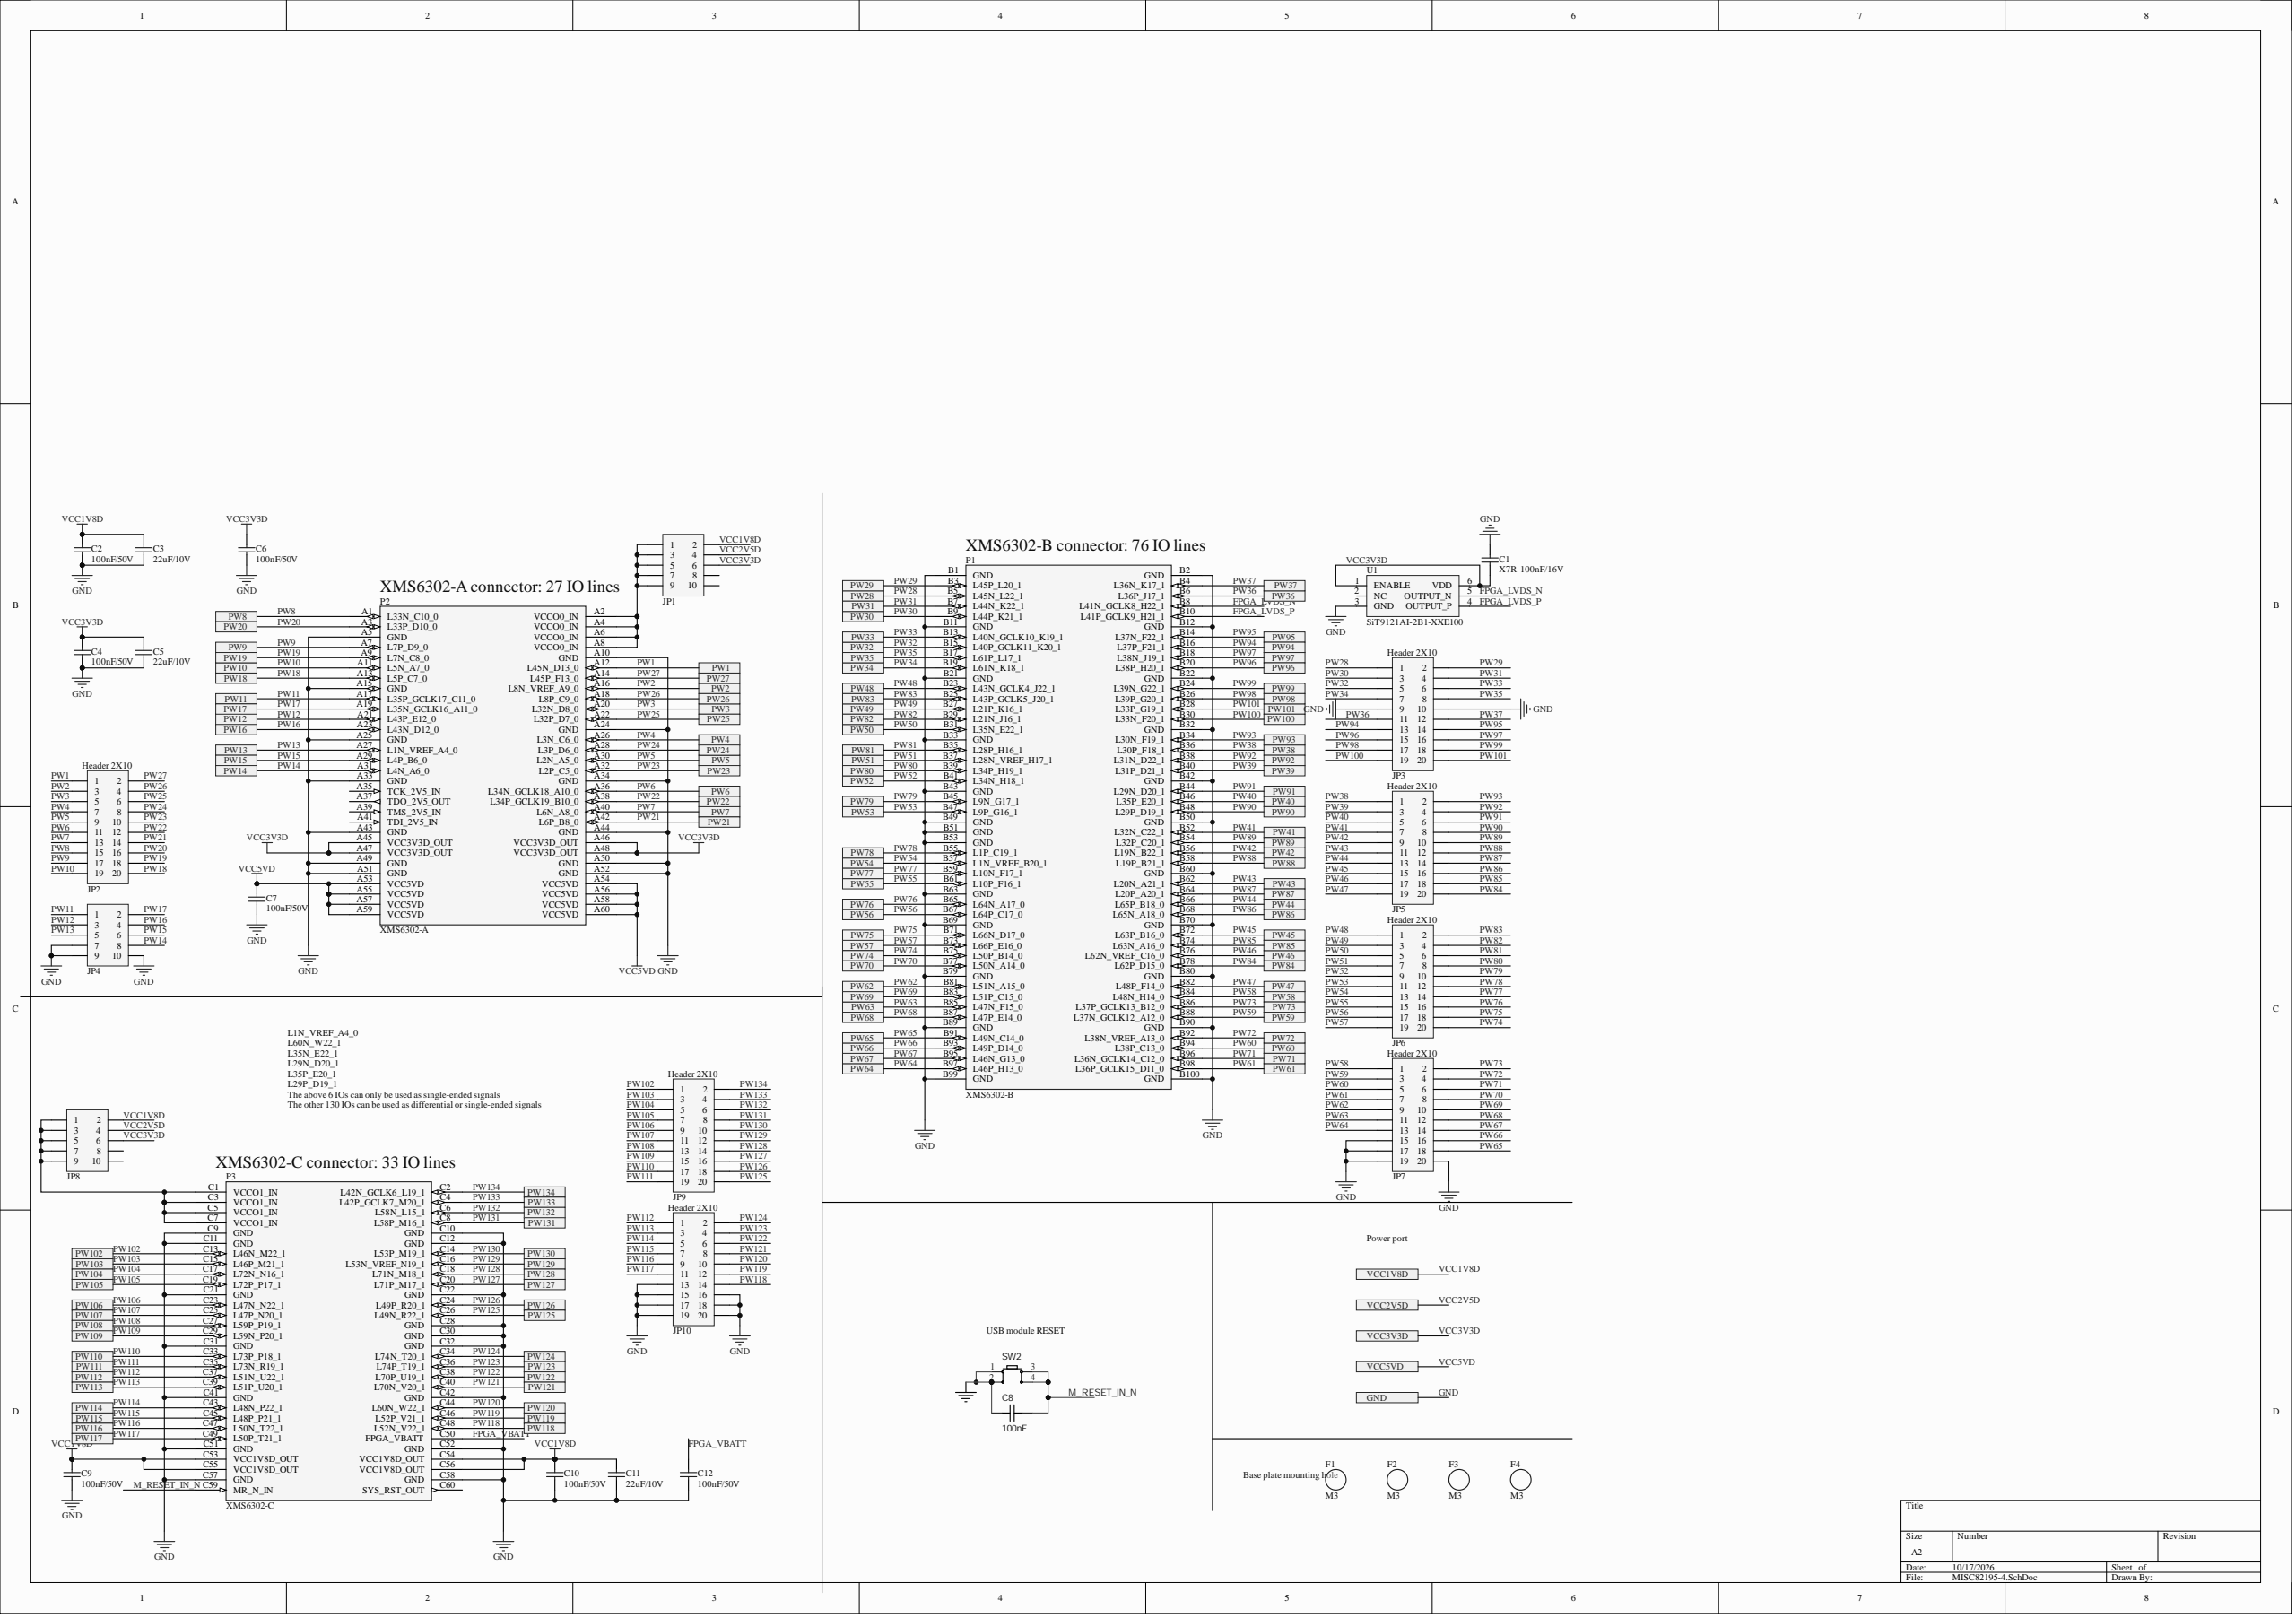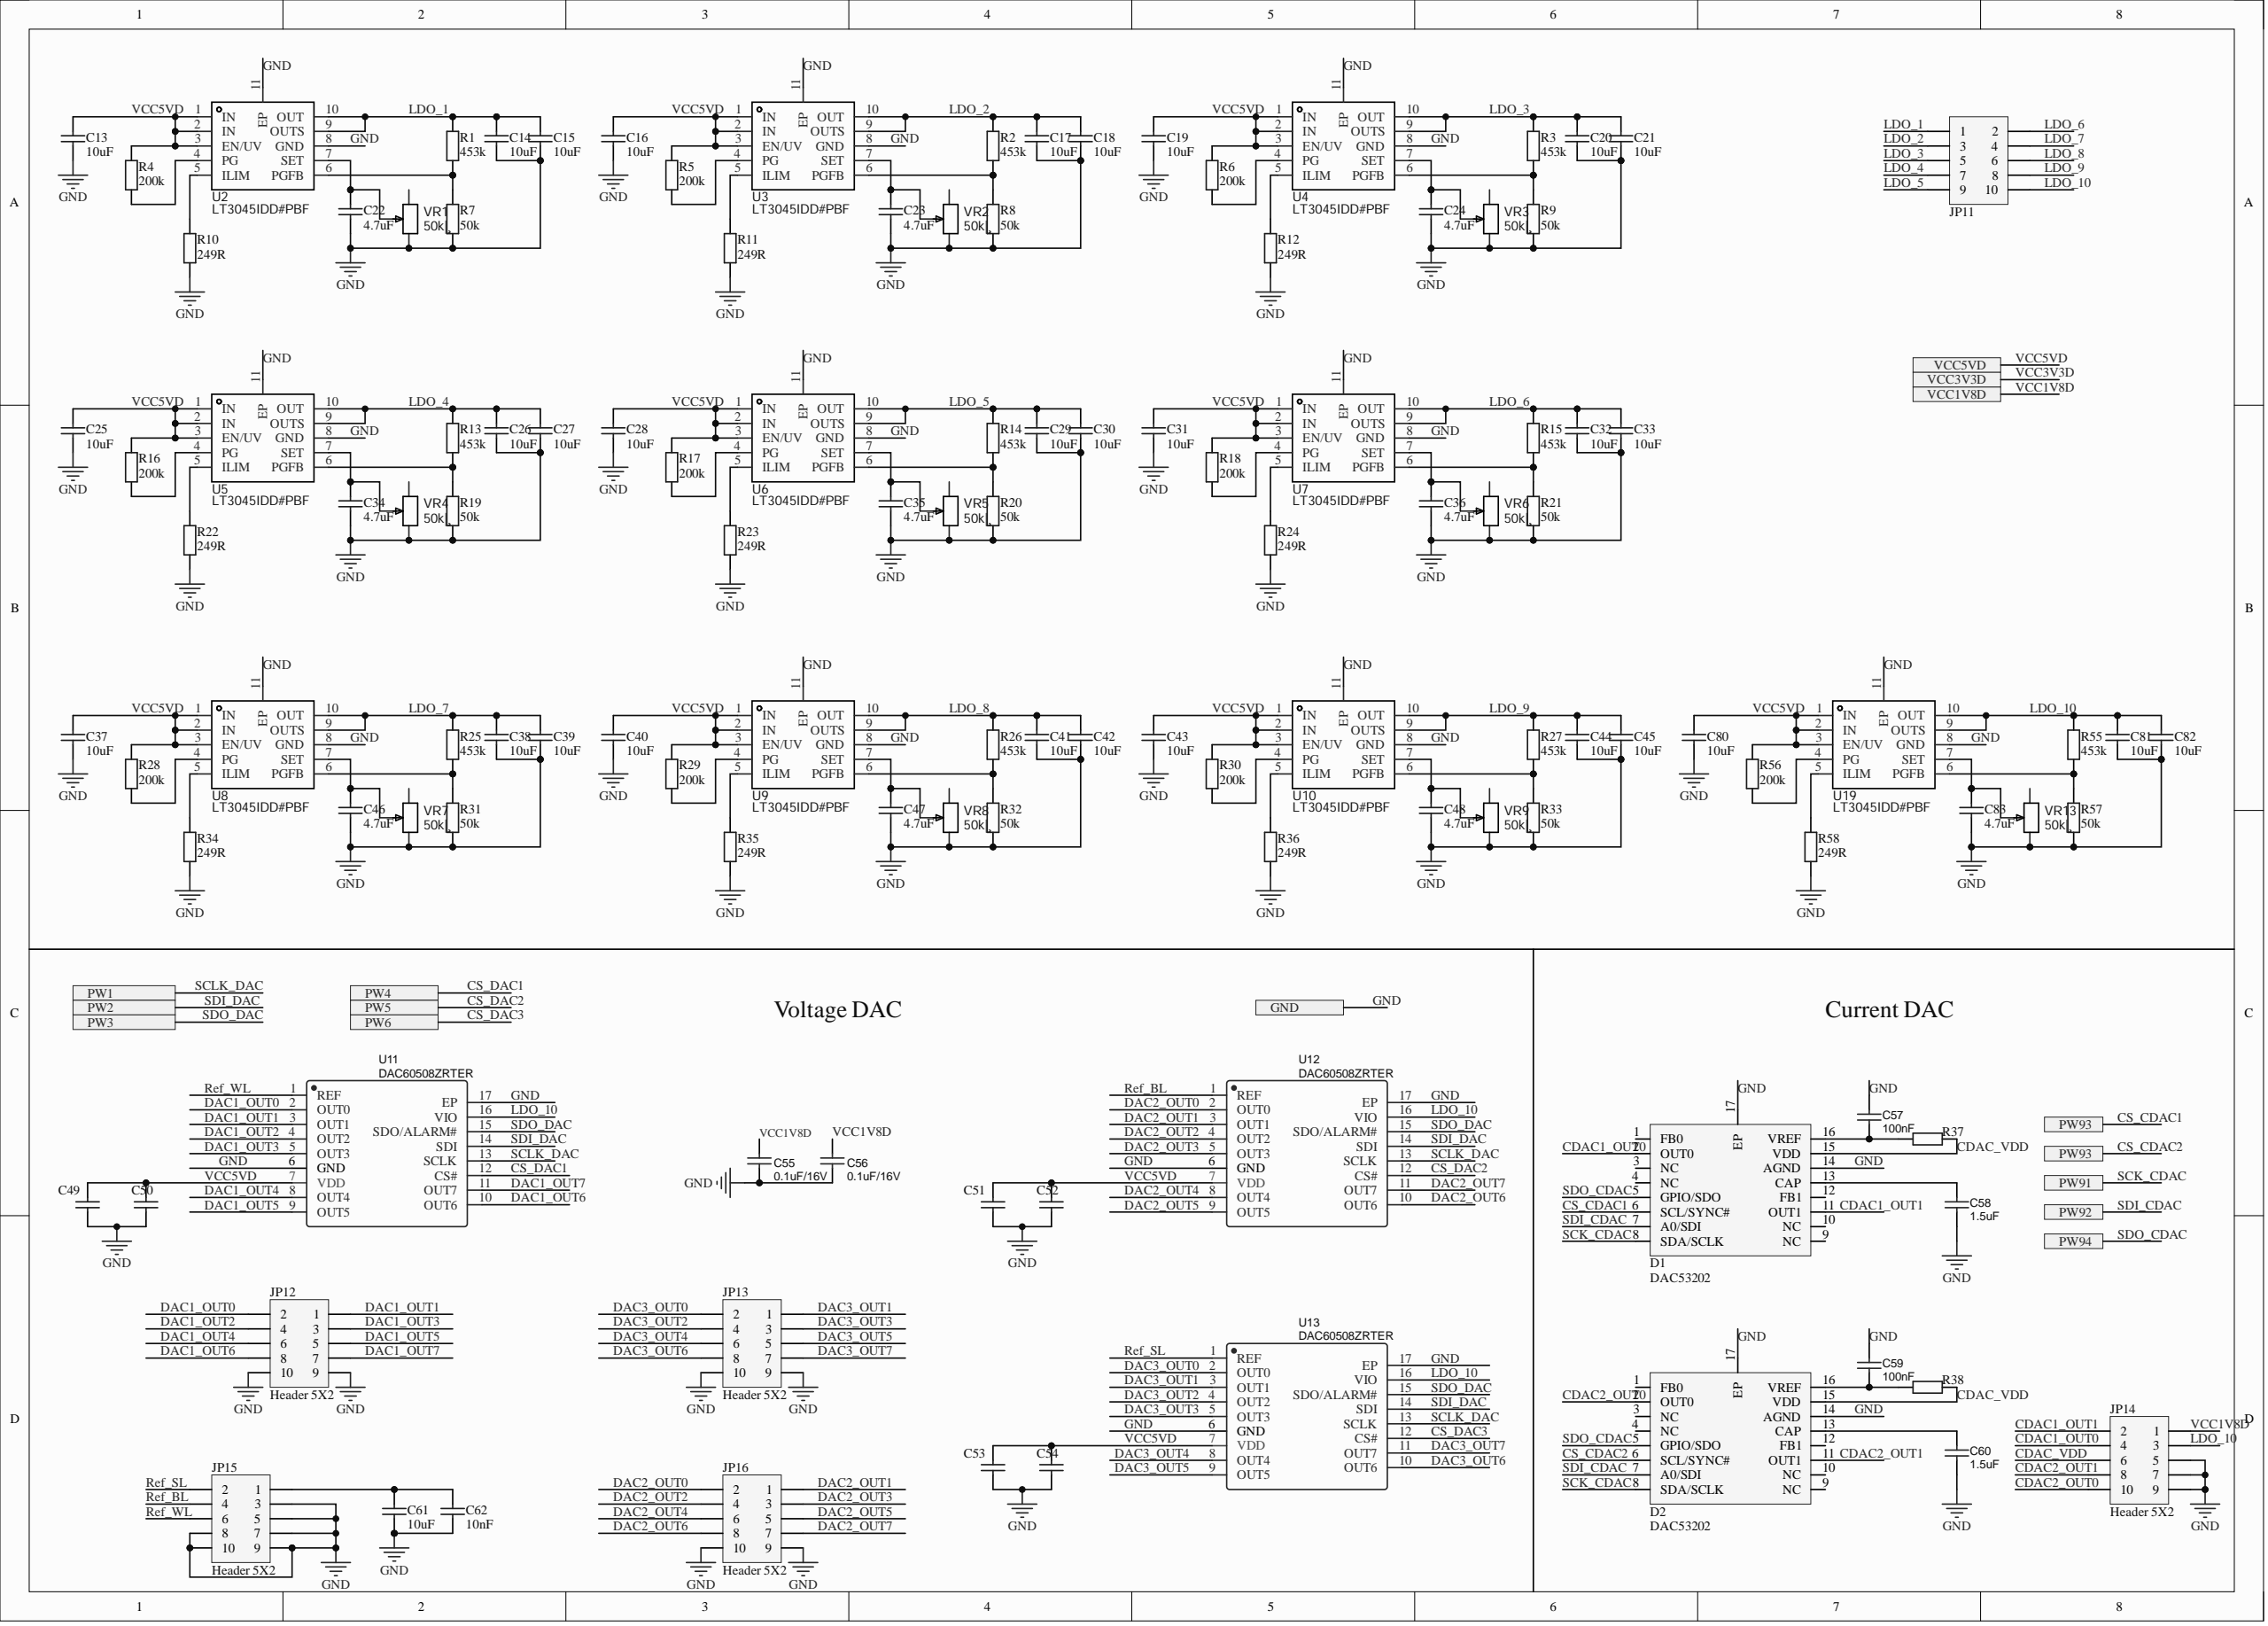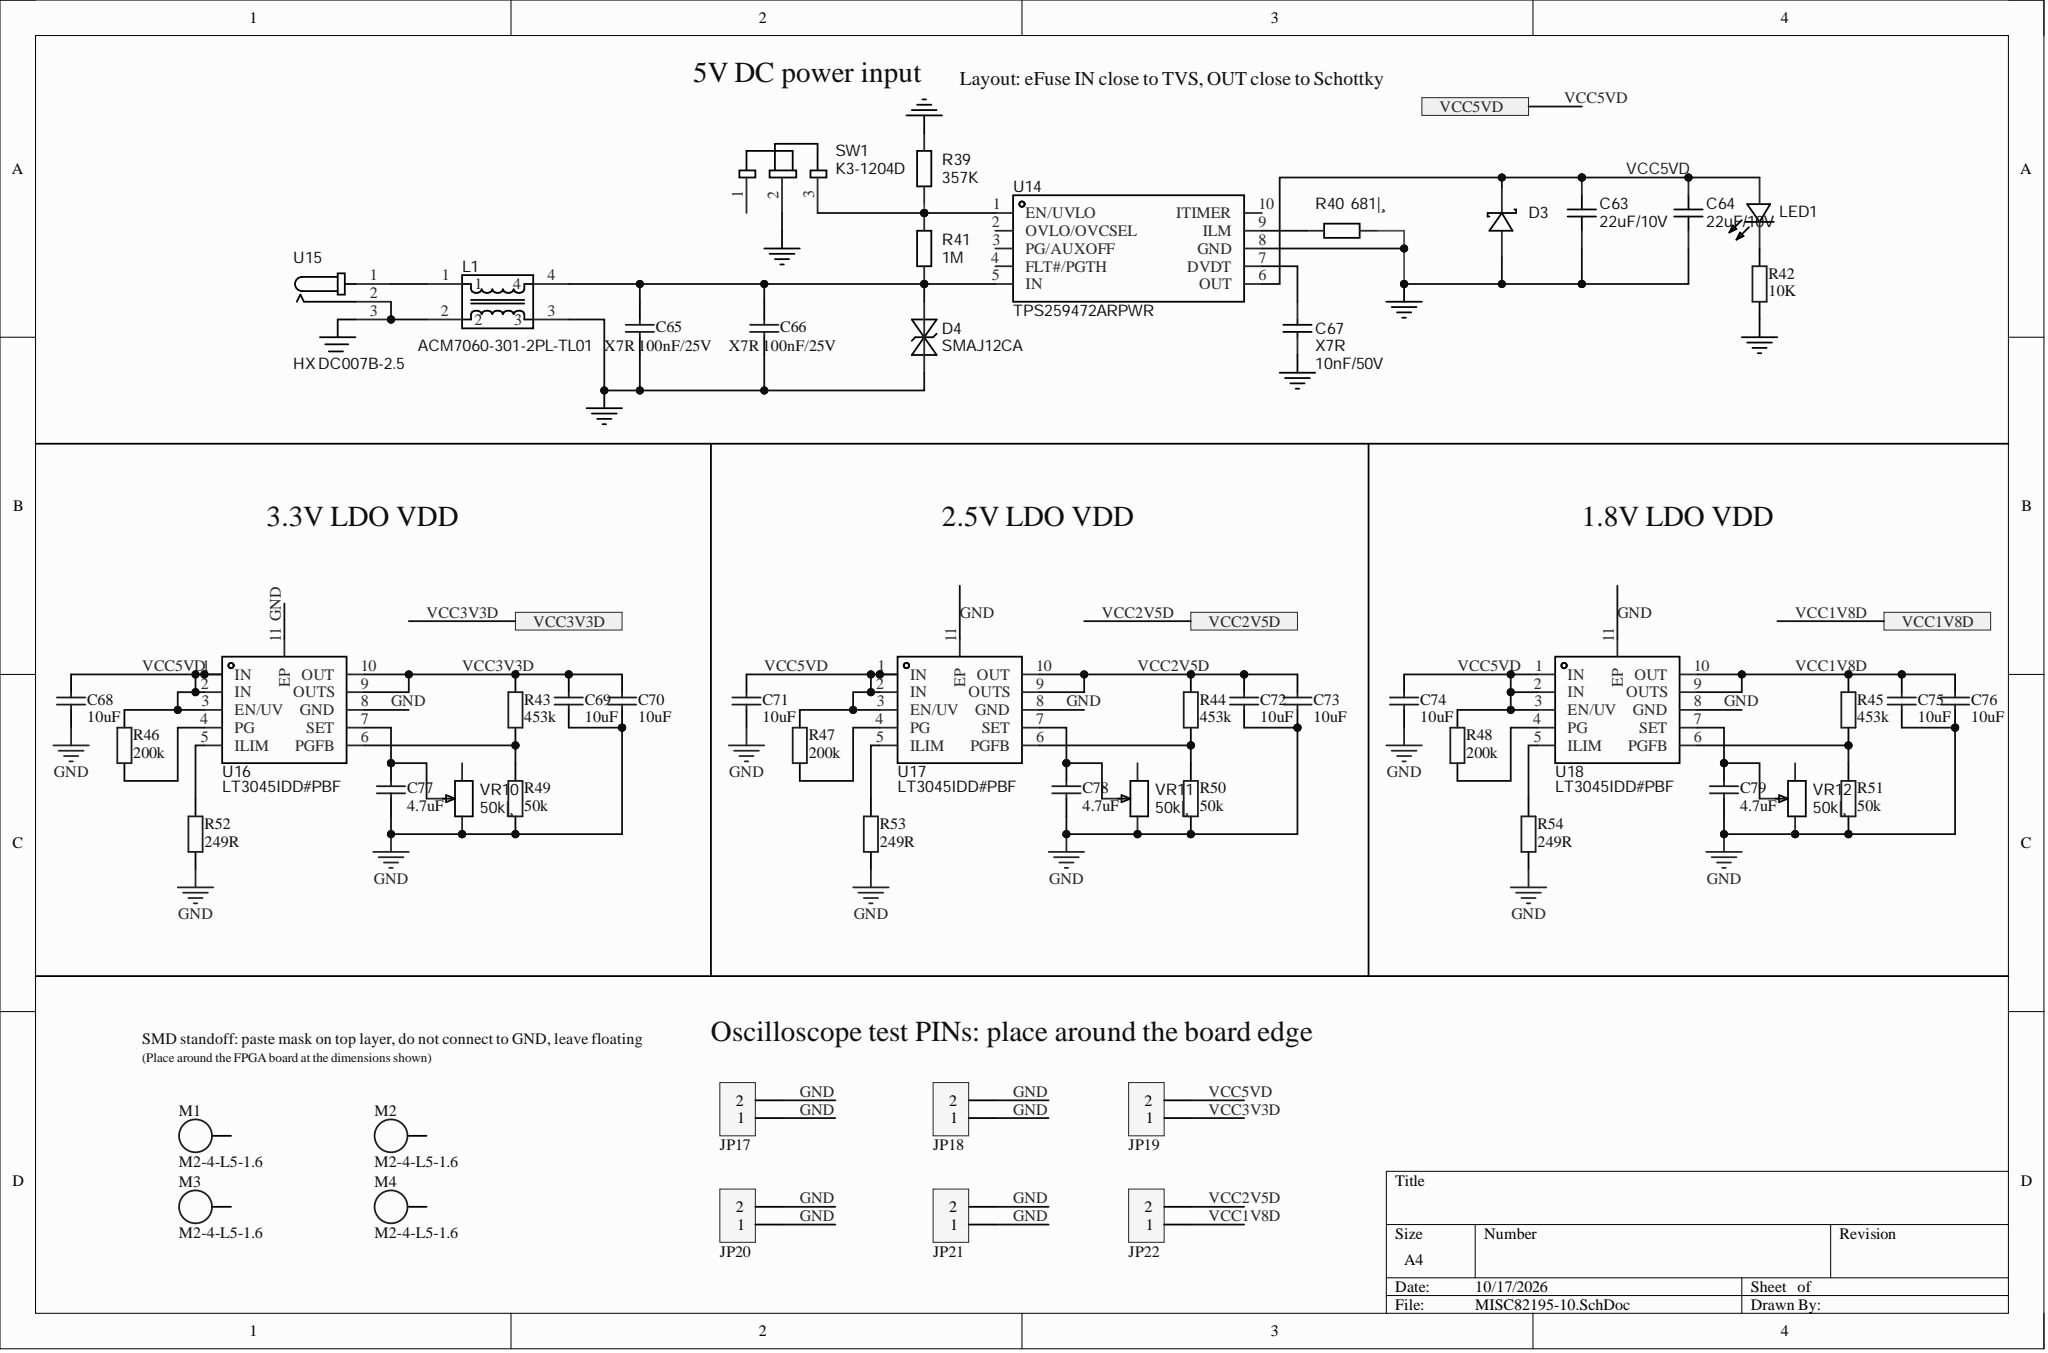Circuit board | Altium Designer | 214 parts | 251 nets
Bill of materials:
Comment,Description,Designator,Footprint,LibRef,Quantity
"X7R  100nF/16V","SMD capacitor","C1","C0603","C","1"
"100nF/50V","SMD capacitor","C2, C4, C6, C7, C9, C10, C12","C0603","C","7"
"22uF/10V","SMD capacitor, [NoValue]","C3, C5, C11, C63, C64","C0603","C, CL21A226MAQNNNE","5"
"100nF","[NoValue], SMD capacitor","C8, C50, C52, C54, C57, C59","C0603","CC0603KRX7R9BB104, C, 1uF","6"
"10uF","SMD capacitor","C13, C14, C15, C16, C17, C18, C19, C20, C21, C25, C26, C27, C28, C29, C30, C31, C32, C33, C37, C38, C39, C40, C41, C42, C43, C44, C45, C49, C51, C53, C61, C68, C69, C70, C71, C72, C73, C74, C75, C76, C80, C81, C82","C0603","C","43"
"4.7uF","SMD capacitor","C22, C23, C24, C34, C35, C36, C46, C47, C48, C77, C78, C79, C83","C0603","C","13"
"0.1uF/16V","","C55, C56","C0603","10nF","2"
"1.5uF","","C58, C60","C0603","1uF","2"
"10nF","SMD capacitor","C62","C0603","C","1"
"X7R 100nF/25V","SMD capacitor","C65, C66","C0603","C","2"
"X7R","","C67","C0603","CC0603KRX7R9BB103","1"
"DAC53202","","D1, D2","WQFN-16(3x3)","DAC53202","2"
"VS-10BQ015HM3/5BT","","D3","SMB_L4.6-W3.6-LS5.3-RD","VS-10BQ015HM3/5BT","1"
"SMAJ12CA","","D4","SMA_L4.2-W2.7-LS5.0-BI","SMAJ12CA_C908818","1"
"M3","Standoff hole","F1, F2, F3, F4","M3","M3","4"
"Header 5X2","5*2P connector","JP1, JP4, JP8, JP11, JP12, JP13, JP14, JP15, JP16","HDR2.54-LI-2x5P","Header 5X2","9"
"Header 2X10","10*2P connector","JP2, JP3, JP5, JP6, JP7, JP9, JP10","HDR2.54-LI-2x10P","Header 10X2","7"
"HDR-1X2","2P connector","JP17, JP18, JP19, JP20, JP21, JP22","HDR2.54-LI-2P","Header 2","6"
"ACM7060-301-2PL-TL01","","L1","FILTER-SMD_4P-L7.0-W6.0-TL_SMCM7060","ACM7060-301-2PL-TL01","1"
"NCD0805G1","","LED1","LED0805-R-RD","NCD0805G1","1"
"M2-4-L5-1.6","SMD standoff","M1, M2, M3, M4","M2.9","M2","4"
"XMS6302-B","","P1","XMS6302-B","XMS6302-B","1"
"XMS6302-A","","P2","XMS6302-A","XMS6302-A","1"
"XMS6302-C","","P3","XMS6302-C","XMS6302-C","1"
"453k","SMD resistor","R1, R2, R3, R13, R14, R15, R25, R26, R27, R43, R44, R45, R55","R0603","R","13"
"200k","SMD resistor","R4, R5, R6, R16, R17, R18, R28, R29, R30, R46, R47, R48, R56","R0603","R","13"
"50k","SMD resistor","R7, R8, R9, R19, R20, R21, R31, R32, R33, R49, R50, R51, R57","R0603","R","13"
"249R","SMD resistor","R10, R11, R12, R22, R23, R24, R34, R35, R36, R52, R53, R54, R58","R0603","R","13"
"10K","SMD resistor","R37, R38, R42","R0603","R","3"
"357K","","R39","R0603","Res_0603","1"
"681|¸","","R40","R0603","CR0805F681RP05Z","1"
"1M","","R41","R0603","Res_0603","1"
"K3-1204D","","SW1","SW-TH_K3-1204D","K3-1204D","1"
"Key_SMD_6x6x6.5","","SW2","SW-SMD_4P-L6.0-W6.0-P4.50-LS9.0-2","Key_SMD_6x6x6.5","1"
"SiT9121AI-2B1-XXE100","100MHz oscillator","U1","3225-6p","SiT9121AI","1"
"LT3045IDD#PBF","","U2, U3, U4, U5, U6, U7, U8, U9, U10, U16, U17, U18, U19","DFN-10_L3.0-W3.0-P0.50-BL-EP-3","LT3045IDD#PBF","13"
"DAC60508ZRTER","","U11, U12, U13","WQFN-16_L3.0-W3.0-P0.50-BL-EP0.8","DAC60508ZRTER","3"
"TPS259472ARPWR","","U14","VQFN-10_L2.0-W2.0-P0.45-TL","TPS259472ARPWR","1"
"HX DC007B-2.5","","U15","DC-IN-TH_HX-DC007B-2.5","HX DC007B-2.5","1"
"50k|¸","","VR1, VR2, VR3, VR4, VR5, VR6, VR7, VR8, VR9, VR10, VR11, VR12, VR13","RES-ADJ-SMD_3224W","3224W-1-503E","13"
Netlist (Protel format):
[
C1
C0603
X7R  100nF/16V



]
[
C2
C0603
100nF/50V



]
[
C3
C0603
22uF/10V



]
[
C4
C0603
100nF/50V



]
[
C5
C0603
22uF/10V



]
[
C6
C0603
100nF/50V



]
[
C7
C0603
100nF/50V



]
[
C8
C0603
100nF



]
[
C9
C0603
100nF/50V



]
[
C10
C0603
100nF/50V



]
[
C11
C0603
22uF/10V



]
[
C12
C0603
100nF/50V



]
[
C13
C0603
10uF



]
[
C14
C0603
10uF



]
[
C15
C0603
10uF



]
[
C16
C0603
10uF



]
[
C17
C0603
10uF



]
[
C18
C0603
10uF



]
[
C19
C0603
10uF



]
[
C20
C0603
10uF



]
[
C21
C0603
10uF



]
[
C22
C0603
4.7uF



]
[
C23
C0603
4.7uF



]
[
C24
C0603
4.7uF



]
[
C25
C0603
10uF



]
[
C26
C0603
10uF



]
[
C27
C0603
10uF



]
[
C28
C0603
10uF



]
[
C29
C0603
10uF



]
[
C30
C0603
10uF



]
[
C31
C0603
10uF



]
[
C32
C0603
10uF



]
[
C33
C0603
10uF



]
[
C34
C0603
4.7uF



]
[
C35
C0603
4.7uF



]
[
C36
C0603
4.7uF



]
[
C37
C0603
10uF



]
[
C38
C0603
10uF



]
[
C39
C0603
10uF



]
[
C40
C0603
10uF



]
[
C41
C0603
10uF



]
[
C42
C0603
10uF



]
[
C43
C0603
10uF



]
[
C44
C0603
10uF



]
[
C45
C0603
10uF



]
[
C46
C0603
4.7uF



]
[
C47
C0603
4.7uF



]
[
C48
C0603
4.7uF



]
[
C49
C0603
10uF



]
[
C50
C0603
100nF



]
[
C51
C0603
10uF



]
[
C52
C0603
100nF



]
[
C53
C0603
10uF



]
[
C54
C0603
100nF



]
[
C55
C0603
0.1uF/16V



]
[
C56
C0603
0.1uF/16V



]
[
C57
C0603
100nF



]
[
C58
C0603
1.5uF



]
[
C59
C0603
100nF



]
[
C60
C0603
1.5uF



]
[
C61
C0603
10uF



]
[
C62
C0603
10nF



]
[
C63
C0603
22uF/10V



]
[
C64
C0603
22uF/10V



]
[
C65
C0603
X7R 100nF/25V



]
[
C66
C0603
X7R 100nF/25V



]
[
C67
C0603
X7R



]
[
C68
C0603
10uF



]
[
C69
C0603
10uF



]
[
C70
C0603
10uF



]
[
C71
C0603
10uF



]
[
C72
C0603
10uF



]
[
C73
C0603
10uF



]
[
C74
C0603
10uF



]
[
C75
C0603
10uF



]
[
C76
C0603
10uF



]
[
C77
C0603
4.7uF



]
[
C78
C0603
4.7uF



]
[
C79
C0603
4.7uF



]
[
C80
C0603
10uF



]
[
C81
C0603
10uF



]
[
C82
C0603
10uF



]
[
C83
C0603
4.7uF



]
[
D1
WQFN-16(3x3)
DAC53202



]
[
D2
WQFN-16(3x3)
DAC53202



]
[
D3
SMB_L4.6-W3.6-LS5.3-RD
VS-10BQ015HM3/5BT



]
[
D4
SMA_L4.2-W2.7-LS5.0-BI
SMAJ12CA



]
[
F1
M3
M3



]
[
F2
M3
M3



]
[
F3
M3
M3



]
[
F4
M3
M3



]
[
JP1
HDR2.54-LI-2x5P
Header 5X2



]
[
JP2
HDR2.54-LI-2x10P
Header 2X10



]
[
JP3
HDR2.54-LI-2x10P
Header 2X10



]
[
JP4
HDR2.54-LI-2x5P
Header 5X2



]
[
JP5
HDR2.54-LI-2x10P
Header 2X10



]
[
JP6
HDR2.54-LI-2x10P
Header 2X10



]
[
JP7
HDR2.54-LI-2x10P
Header 2X10



]
[
JP8
HDR2.54-LI-2x5P
Header 5X2



]
[
JP9
HDR2.54-LI-2x10P
Header 2X10



]
[
JP10
HDR2.54-LI-2x10P
Header 2X10



]
[
JP11
HDR2.54-LI-2x5P
Header 5X2



]
[
JP12
HDR2.54-LI-2x5P
Header 5X2



]
[
JP13
HDR2.54-LI-2x5P
Header 5X2



]
[
JP14
HDR2.54-LI-2x5P
Header 5X2



]
[
JP15
HDR2.54-LI-2x5P
Header 5X2



]
[
JP16
HDR2.54-LI-2x5P
Header 5X2



]
[
JP17
HDR2.54-LI-2P
HDR-1X2



]
[
JP18
HDR2.54-LI-2P
HDR-1X2



]
[
JP19
HDR2.54-LI-2P
HDR-1X2



]
[
JP20
HDR2.54-LI-2P
HDR-1X2



]
[
JP21
HDR2.54-LI-2P
HDR-1X2



]
[
JP22
HDR2.54-LI-2P
HDR-1X2



]
[
L1
FILTER-SMD_4P-L7.0-W6.0-TL_SMCM7060
ACM7060-301-2PL-TL01



]
[
LED1
LED0805-R-RD
NCD0805G1



]
[
M1
M2.9
M2-4-L5-1.6



]
[
M2
M2.9
M2-4-L5-1.6



]
[
M3
M2.9
M2-4-L5-1.6



]
[
M4
M2.9
M2-4-L5-1.6



]
[
P1
XMS6302-B
XMS6302-B



]
[
P2
XMS6302-A
XMS6302-A



]
[
P3
XMS6302-C
XMS6302-C



]
[
R1
R0603
453k



]
[
R2
R0603
453k



]
[
R3
R0603
453k



]
[
R4
R0603
200k



]
[
R5
R0603
200k



]
[
R6
R0603
200k



]
[
R7
R0603
50k



]
[
R8
R0603
50k



]
[
R9
R0603
50k



]
[
R10
R0603
249R



]
[
R11
R0603
249R



]
[
R12
R0603
249R



]
[
R13
R0603
453k



]
[
R14
R0603
453k



]
[
R15
R0603
453k



]
[
R16
R0603
200k



]
[
R17
R0603
200k



]
[
R18
R0603
200k



]
[
R19
R0603
50k



]
[
R20
R0603
50k



]
[
R21
R0603
50k



]
[
R22
R0603
249R



]
[
R23
R0603
249R



]
[
R24
R0603
249R



]
[
R25
R0603
453k



]
[
R26
R0603
453k



]
[
R27
R0603
453k



]
[
R28
R0603
200k



]
[
R29
R0603
200k



]
[
R30
R0603
200k



]
[
R31
R0603
50k



]
[
R32
R0603
50k



]
[
R33
R0603
50k



]
[
R34
R0603
249R



]
[
R35
R0603
249R



]
[
R36
R0603
249R



]
[
R37
R0603
10K



]
[
R38
R0603
10K



]
[
R39
R0603
357K



]
[
R40
R0603
681|¸



]
[
R41
R0603
1M



]
[
R42
R0603
10K



]
[
R43
R0603
453k



]
[
R44
R0603
453k



]
[
R45
R0603
453k



]
[
R46
R0603
200k



]
[
R47
R0603
200k



]
[
R48
R0603
200k



]
[
R49
R0603
50k



]
[
R50
R0603
50k



]
[
R51
R0603
50k



]
[
R52
R0603
249R



]
[
R53
R0603
249R



]
[
R54
R0603
249R



]
[
R55
R0603
453k



]
[
R56
R0603
200k



]
[
R57
R0603
50k



]
[
R58
R0603
249R



]
[
SW1
SW-TH_K3-1204D
K3-1204D



]
[
SW2
SW-SMD_4P-L6.0-W6.0-P4.50-LS9.0-2
Key_SMD_6x6x6.5



]
[
U1
3225-6p
SiT9121AI-2B1-XXE100



]
[
U2
DFN-10_L3.0-W3.0-P0.50-BL-EP-3
LT3045IDD#PBF



]
[
U3
DFN-10_L3.0-W3.0-P0.50-BL-EP-3
LT3045IDD#PBF



]
[
U4
DFN-10_L3.0-W3.0-P0.50-BL-EP-3
LT3045IDD#PBF



]
[
U5
DFN-10_L3.0-W3.0-P0.50-BL-EP-3
LT3045IDD#PBF



]
[
U6
DFN-10_L3.0-W3.0-P0.50-BL-EP-3
LT3045IDD#PBF



]
[
U7
DFN-10_L3.0-W3.0-P0.50-BL-EP-3
LT3045IDD#PBF



]
[
U8
DFN-10_L3.0-W3.0-P0.50-BL-EP-3
LT3045IDD#PBF



]
[
U9
DFN-10_L3.0-W3.0-P0.50-BL-EP-3
LT3045IDD#PBF



]
[
U10
DFN-10_L3.0-W3.0-P0.50-BL-EP-3
LT3045IDD#PBF



]
[
U11
WQFN-16_L3.0-W3.0-P0.50-BL-EP0.8
DAC60508ZRTER



]
[
U12
WQFN-16_L3.0-W3.0-P0.50-BL-EP0.8
DAC60508ZRTER



]
[
U13
WQFN-16_L3.0-W3.0-P0.50-BL-EP0.8
DAC60508ZRTER



]
[
U14
VQFN-10_L2.0-W2.0-P0.45-TL
TPS259472ARPWR



]
[
U15
DC-IN-TH_HX-DC007B-2.5
HX DC007B-2.5



]
[
U16
DFN-10_L3.0-W3.0-P0.50-BL-EP-3
LT3045IDD#PBF



]
[
U17
DFN-10_L3.0-W3.0-P0.50-BL-EP-3
LT3045IDD#PBF



]
[
U18
DFN-10_L3.0-W3.0-P0.50-BL-EP-3
LT3045IDD#PBF



]
[
U19
DFN-10_L3.0-W3.0-P0.50-BL-EP-3
LT3045IDD#PBF



]
[
VR1
RES-ADJ-SMD_3224W
50k|¸



]
[
VR2
RES-ADJ-SMD_3224W
50k|¸



]
[
VR3
RES-ADJ-SMD_3224W
50k|¸



]
[
VR4
RES-ADJ-SMD_3224W
50k|¸



]
[
VR5
RES-ADJ-SMD_3224W
50k|¸



]
[
VR6
RES-ADJ-SMD_3224W
50k|¸



]
[
VR7
RES-ADJ-SMD_3224W
50k|¸



]
[
VR8
RES-ADJ-SMD_3224W
50k|¸



]
[
VR9
RES-ADJ-SMD_3224W
50k|¸



]
[
VR10
RES-ADJ-SMD_3224W
50k|¸



]
[
VR11
RES-ADJ-SMD_3224W
50k|¸



]
[
VR12
RES-ADJ-SMD_3224W
50k|¸



]
[
VR13
RES-ADJ-SMD_3224W
50k|¸



]
(
VCC5VD
C7-2
C13-2
C16-2
C19-2
C25-2
C28-2
C31-2
C37-2
C40-2
C43-2
C49-2
C50-2
C51-2
C52-2
C53-2
C54-2
C63-2
C64-2
C68-2
C71-2
C74-2
C80-2
D3-1
JP19-2
LED1-1
P2-A53
P2-A54
P2-A55
P2-A56
P2-A57
P2-A58
P2-A59
P2-A60
R4-2
R5-2
R6-2
R16-2
R17-2
R18-2
R28-2
R29-2
R30-2
R46-2
R47-2
R48-2
R56-2
U2-1
U2-2
U2-3
U3-1
U3-2
U3-3
U4-1
U4-2
U4-3
U5-1
U5-2
U5-3
U6-1
U6-2
U6-3
U7-1
U7-2
U7-3
U8-1
U8-2
U8-3
U9-1
U9-2
U9-3
U10-1
U10-2
U10-3
U11-7
U12-7
U13-7
U14-6
U16-1
U16-2
U16-3
U17-1
U17-2
U17-3
U18-1
U18-2
U18-3
U19-1
U19-2
U19-3
)
(
VCC3V3D
C1-1
C4-2
C5-2
C6-2
C69-2
C70-2
JP1-6
JP8-6
JP19-1
P2-A45
P2-A46
P2-A47
P2-A48
R43-2
U1-1
U1-6
U16-9
U16-10
)
(
VCC2V5D
C72-2
C73-2
JP1-4
JP8-4
JP22-2
R44-2
U17-9
U17-10
)
(
VCC1V8D
C2-2
C3-2
C9-2
C10-2
C11-2
C55-2
C56-2
C75-2
C76-2
JP1-2
JP8-2
JP14-1
JP22-1
P3-C53
P3-C54
P3-C55
P3-C56
R45-2
U18-9
U18-10
)
(
Ref_WL
JP15-6
U11-1
)
(
Ref_SL
JP15-2
U13-1
)
(
Ref_BL
JP15-4
U12-1
)
(
PW134
JP9-2
P3-C2
)
(
PW133
JP9-4
P3-C4
)
(
PW132
JP9-6
P3-C6
)
(
PW131
JP9-8
P3-C8
)
(
PW130
JP9-10
P3-C14
)
(
PW129
JP9-12
P3-C16
)
(
PW128
JP9-14
P3-C18
)
(
PW127
JP9-16
P3-C20
)
(
PW126
JP9-18
P3-C24
)
(
PW125
JP9-20
P3-C26
)
(
PW124
JP10-2
P3-C34
)
(
PW123
JP10-4
P3-C36
)
(
PW122
JP10-6
P3-C38
)
(
PW121
JP10-8
P3-C40
)
(
PW120
JP10-10
P3-C44
)
(
PW119
JP10-12
P3-C46
)
(
PW118
JP10-14
P3-C48
)
(
PW117
JP10-11
P3-C49
)
(
PW116
JP10-9
P3-C47
)
(
PW115
JP10-7
P3-C45
)
(
PW114
JP10-5
P3-C43
)
(
PW113
JP10-3
P3-C39
)
(
PW112
JP10-1
P3-C37
)
(
PW111
JP9-19
P3-C35
)
(
PW110
JP9-17
P3-C33
)
(
PW109
JP9-15
P3-C29
)
(
PW108
JP9-13
P3-C27
)
(
PW107
JP9-11
P3-C25
)
(
PW106
JP9-9
P3-C23
)
(
PW105
JP9-7
P3-C19
)
(
PW104
JP9-5
P3-C17
)
(
PW103
JP9-3
P3-C15
)
(
PW102
JP9-1
P3-C13
)
(
PW101
JP3-20
P1-B28
)
(
PW100
JP3-19
P1-B30
)
(
PW99
JP3-18
P1-B24
)
(
PW98
JP3-17
P1-B26
)
(
PW97
JP3-16
P1-B18
)
(
PW96
JP3-15
P1-B20
)
(
PW95
JP3-14
P1-B14
)
(
PW94
D1-5
D2-5
JP3-13
P1-B16
)
(
PW92
D1-7
D2-7
JP5-4
P1-B38
)
(
PW91
D1-8
D2-8
JP5-6
P1-B44
)
(
PW90
JP5-8
P1-B48
)
(
PW89
JP5-10
P1-B54
)
(
PW88
JP5-12
P1-B58
)
(
PW87
JP5-14
P1-B64
)
(
PW86
JP5-16
P1-B68
)
(
PW85
JP5-18
P1-B74
)
(
PW84
JP5-20
P1-B78
)
(
PW83
JP6-2
P1-B25
)
(
PW82
JP6-4
P1-B29
)
(
PW81
JP6-6
P1-B35
)
(
PW80
JP6-8
P1-B39
)
(
PW79
JP6-10
P1-B45
)
(
PW78
JP6-12
P1-B55
)
(
PW77
JP6-14
P1-B59
)
(
PW76
JP6-16
P1-B65
)
(
PW75
JP6-18
P1-B71
)
(
PW74
JP6-20
P1-B75
)
(
PW73
JP7-2
P1-B86
)
(
PW72
JP7-4
P1-B92
)
(
PW71
JP7-6
P1-B96
)
(
PW70
JP7-8
P1-B77
)
(
PW69
JP7-10
P1-B83
)
(
PW68
JP7-12
P1-B87
)
(
PW67
JP7-14
P1-B95
)
(
PW66
JP7-16
P1-B93
)
(
PW65
JP7-18
P1-B91
)
(
PW64
JP7-13
P1-B97
)
(
PW63
JP7-11
P1-B85
)
(
PW62
JP7-9
P1-B81
)
(
PW61
JP7-7
P1-B98
)
(
PW60
JP7-5
P1-B94
)
(
PW59
JP7-3
P1-B88
)
(
PW58
JP7-1
P1-B84
)
(
PW57
JP6-19
P1-B73
)
(
PW56
JP6-17
P1-B67
)
(
PW55
JP6-15
P1-B61
)
(
PW54
JP6-13
P1-B57
)
(
PW53
JP6-11
P1-B47
)
(
PW52
JP6-9
P1-B41
)
(
PW51
JP6-7
P1-B37
)
(
PW50
JP6-5
P1-B31
)
(
PW49
JP6-3
P1-B27
)
(
PW48
JP6-1
P1-B23
)
(
PW47
JP5-19
P1-B82
)
(
PW46
JP5-17
P1-B76
)
(
PW45
JP5-15
P1-B72
)
(
PW44
JP5-13
P1-B66
)
(
PW43
JP5-11
P1-B62
)
(
PW42
JP5-9
P1-B56
)
(
PW41
JP5-7
P1-B52
)
(
PW40
JP5-5
P1-B46
)
(
PW39
JP5-3
P1-B40
)
(
PW38
JP5-1
P1-B36
)
(
PW37
JP3-12
P1-B4
)
(
PW36
JP3-11
P1-B6
)
(
PW35
JP3-8
P1-B17
)
(
PW34
JP3-7
P1-B19
)
(
PW33
JP3-6
P1-B13
)
(
PW32
JP3-5
P1-B15
)
(
PW31
JP3-4
P1-B7
)
(
PW30
JP3-3
P1-B9
)
(
PW29
JP3-2
P1-B3
)
(
PW28
JP3-1
P1-B5
)
(
PW27
JP2-2
P2-A14
)
(
PW26
JP2-4
P2-A18
)
(
PW25
JP2-6
P2-A22
)
(
PW24
JP2-8
P2-A28
)
(
PW23
JP2-10
P2-A32
)
(
PW22
JP2-12
P2-A38
)
(
PW21
JP2-14
P2-A42
)
(
PW20
JP2-16
P2-A3
)
(
PW19
JP2-18
P2-A9
)
(
PW18
JP2-20
P2-A13
)
(
PW17
JP4-2
P2-A19
)
(
PW16
JP4-4
P2-A23
)
(
PW15
JP4-6
P2-A29
)
(
PW14
JP4-8
P2-A31
)
(
PW13
JP4-5
P2-A27
)
(
PW12
JP4-3
P2-A21
)
(
PW11
JP4-1
P2-A17
)
(
PW10
JP2-19
P2-A11
)
(
PW9
JP2-17
P2-A7
)
(
PW8
JP2-15
P2-A1
)
(
PW7
JP2-13
P2-A40
)
(
PW3
JP2-5
P2-A20
U11-15
U12-15
U13-15
)
(
PW2
JP2-3
P2-A16
U11-14
U12-14
U13-14
)
(
PW1
JP2-1
P2-A12
U11-13
U12-13
U13-13
)
(
NetR58_2
R58-2
U19-5
)
(
NetR56_1
R56-1
U19-4
)
(
NetR55_1
R55-1
R57-2
U19-6
)
(
NetR54_2
R54-2
U18-5
)
(
NetR53_2
R53-2
U17-5
)
(
NetR52_2
R52-2
U16-5
)
(
NetR48_1
R48-1
U18-4
)
(
NetR47_1
R47-1
U17-4
)
(
NetR46_1
R46-1
U16-4
)
(
NetR45_1
R45-1
R51-2
U18-6
)
(
NetR44_1
R44-1
R50-2
U17-6
)
(
NetR43_1
R43-1
R49-2
U16-6
)
(
NetR40_1
R40-1
U14-9
)
(
NetR39_1
R39-1
R41-2
SW1-3
U14-1
)
(
NetR36_2
R36-2
U10-5
)
(
NetR35_2
R35-2
U9-5
)
(
NetR34_2
R34-2
U8-5
)
(
NetR30_1
R30-1
U10-4
)
(
NetR29_1
R29-1
U9-4
)
(
NetR28_1
R28-1
U8-4
)
(
NetR27_1
R27-1
R33-2
U10-6
)
(
NetR26_1
R26-1
R32-2
U9-6
)
(
NetR25_1
R25-1
R31-2
U8-6
)
(
NetR24_2
R24-2
U7-5
)
(
NetR23_2
R23-2
U6-5
)
(
NetR22_2
R22-2
U5-5
)
(
NetR18_1
R18-1
U7-4
)
(
NetR17_1
R17-1
U6-4
)
(
NetR16_1
R16-1
U5-4
)
(
NetR15_1
R15-1
R21-2
U7-6
)
(
NetR14_1
R14-1
R20-2
U6-6
)
(
NetR13_1
R13-1
R19-2
U5-6
)
(
NetR12_2
R12-2
U4-5
)
(
NetR11_2
R11-2
U3-5
)
(
NetR10_2
R10-2
U2-5
)
(
NetR6_1
R6-1
U4-4
)
(
NetR5_1
R5-1
U3-4
)
(
NetR4_1
R4-1
U2-4
)
(
NetR3_1
R3-1
R9-2
U4-6
)
(
NetR2_1
R2-1
R8-2
U3-6
)
(
NetR1_1
R1-1
R7-2
U2-6
)
(
NetLED1_2
LED1-2
R42-2
)
(
NetL1_2
L1-2
U15-2
U15-3
)
(
NetL1_1
L1-1
U15-1
)
(
NetJP8_1
JP8-1
JP8-3
JP8-5
JP8-7
JP8-9
P3-C1
P3-C3
P3-C5
P3-C7
)
(
NetJP1_1
JP1-1
JP1-3
JP1-5
JP1-7
JP1-9
P2-A2
P2-A4
P2-A6
P2-A8
)
(
NetC83_2
C83-2
U19-7
VR13-2
)
(
NetC79_2
C79-2
U18-7
VR12-2
)
(
NetC78_2
C78-2
U17-7
VR11-2
)
(
NetC77_2
C77-2
U16-7
VR10-2
)
(
NetC67_2
C67-2
U14-7
)
(
NetC65_2
C65-2
C66-2
D4-2
L1-4
R41-1
U14-5
)
(
NetC61_2
C61-2
C62-2
JP15-1
)
(
NetC60_1
C60-1
D2-13
)
(
NetC59_2
C59-2
D2-16
R38-1
)
(
NetC58_1
C58-1
D1-13
)
(
NetC57_2
C57-2
D1-16
R37-1
)
(
NetC48_2
C48-2
U10-7
VR9-2
)
(
NetC47_2
C47-2
U9-7
VR8-2
)
(
NetC46_2
C46-2
U8-7
VR7-2
)
(
NetC36_2
C36-2
U7-7
VR6-2
)
(
NetC35_2
C35-2
U6-7
VR5-2
)
(
NetC34_2
C34-2
U5-7
VR4-2
)
(
NetC24_2
C24-2
U4-7
VR3-2
)
(
NetC23_2
C23-2
U3-7
VR2-2
)
(
NetC22_2
C22-2
U2-7
VR1-2
)
(
M_RESET_IN_N
C8-1
P3-C59
SW2-3
SW2-4
)
(
LDO_10
C81-2
C82-2
JP11-10
JP14-3
R55-2
U11-16
U12-16
U13-16
U19-9
U19-10
)
(
LDO_9
C44-2
C45-2
JP11-8
R27-2
U10-9
U10-10
)
(
LDO_8
C41-2
C42-2
JP11-6
R26-2
U9-9
U9-10
)
(
LDO_7
C38-2
C39-2
JP11-4
R25-2
U8-9
U8-10
)
(
LDO_6
C32-2
C33-2
JP11-2
R15-2
U7-9
U7-10
)
(
LDO_5
C29-2
C30-2
JP11-9
R14-2
U6-9
U6-10
)
(
LDO_4
C26-2
C27-2
JP11-7
R13-2
U5-9
U5-10
)
(
LDO_3
C20-2
C21-2
JP11-5
R3-2
U4-9
U4-10
)
(
LDO_2
C17-2
C18-2
JP11-3
R2-2
U3-9
U3-10
)
(
LDO_1
C14-2
C15-2
JP11-1
R1-2
U2-9
U2-10
)
(
GND
C1-2
C2-1
C3-1
C4-1
C5-1
C6-1
C7-1
C8-2
C9-1
C10-1
C11-1
C12-2
C13-1
C14-1
C15-1
C16-1
C17-1
C18-1
C19-1
C20-1
C21-1
C22-1
C23-1
C24-1
C25-1
C26-1
C27-1
C28-1
C29-1
C30-1
C31-1
C32-1
C33-1
C34-1
C35-1
C36-1
C37-1
C38-1
C39-1
C40-1
C41-1
C42-1
C43-1
C44-1
C45-1
C46-1
C47-1
C48-1
C49-1
C50-1
C51-1
C52-1
C53-1
C54-1
C55-1
C56-1
C57-1
C58-2
C59-1
C60-2
C61-1
C62-1
C63-1
C64-1
C65-1
C66-1
C67-1
C68-1
C69-1
C70-1
C71-1
C72-1
C73-1
C74-1
C75-1
C76-1
C77-1
C78-1
C79-1
C80-1
C81-1
C82-1
C83-1
D1-14
D1-17
D2-14
D2-17
D3-2
D4-1
JP3-9
JP3-10
JP4-7
JP4-9
JP4-10
JP7-15
JP7-17
JP7-19
JP7-20
JP10-13
JP10-15
JP10-16
JP10-17
JP10-18
JP10-19
JP10-20
JP12-9
JP12-10
JP13-9
JP13-10
JP14-5
JP14-7
JP14-9
JP15-3
JP15-5
JP15-7
JP15-8
JP15-9
JP15-10
JP16-9
JP16-10
JP17-1
JP17-2
JP18-1
JP18-2
JP20-1
JP20-2
JP21-1
JP21-2
L1-3
P1-B1
P1-B2
P1-B11
P1-B12
P1-B21
P1-B22
P1-B32
P1-B33
P1-B42
P1-B43
P1-B49
P1-B50
P1-B51
P1-B53
P1-B60
P1-B63
P1-B69
P1-B70
P1-B79
P1-B80
P1-B89
P1-B90
P1-B99
P1-B100
P2-A5
P2-A10
P2-A15
P2-A24
P2-A25
P2-A33
P2-A34
P2-A43
P2-A44
P2-A49
P2-A50
P2-A51
P2-A52
P3-C9
P3-C10
P3-C11
P3-C12
P3-C21
P3-C22
P3-C28
P3-C30
P3-C31
P3-C32
P3-C41
P3-C42
P3-C51
P3-C52
P3-C57
P3-C58
R7-1
R8-1
R9-1
R10-1
R11-1
R12-1
R19-1
R20-1
R21-1
R22-1
R23-1
R24-1
R31-1
R32-1
R33-1
R34-1
R35-1
R36-1
R39-2
R40-2
R42-1
R49-1
R50-1
R51-1
R52-1
R53-1
R54-1
R57-1
R58-1
SW1-2
SW2-1
SW2-2
U1-3
U2-8
U2-11
U3-8
U3-11
U4-8
U4-11
U5-8
U5-11
U6-8
U6-11
U7-8
U7-11
U8-8
U8-11
U9-8
U9-11
U10-8
U10-11
U11-6
U11-17
U12-6
U12-17
U13-6
U13-17
U14-8
U16-8
U16-11
U17-8
U17-11
U18-8
U18-11
U19-8
U19-11
VR1-3
VR2-3
VR3-3
VR4-3
VR5-3
VR6-3
VR7-3
VR8-3
VR9-3
VR10-3
VR11-3
VR12-3
VR13-3
)
(
FPGA_VBATT
C12-1
P3-C50
)
(
FPGA_LVDS_P
P1-B10
U1-4
)
(
FPGA_LVDS_N
P1-B8
U1-5
)
(
DAC3_OUT7
JP13-7
U13-11
)
(
DAC3_OUT6
JP13-8
U13-10
)
(
DAC3_OUT5
JP13-5
U13-9
)
(
DAC3_OUT4
JP13-6
U13-8
)
(
DAC3_OUT3
JP13-3
U13-5
)
(
DAC3_OUT2
JP13-4
U13-4
)
(
DAC3_OUT1
JP13-1
U13-3
)
(
DAC3_OUT0
JP13-2
U13-2
)
(
DAC2_OUT7
JP16-7
U12-11
)
(
DAC2_OUT6
JP16-8
U12-10
)
(
DAC2_OUT5
JP16-5
U12-9
)
(
DAC2_OUT4
JP16-6
U12-8
)
(
DAC2_OUT3
JP16-3
U12-5
)
(
DAC2_OUT2
JP16-4
U12-4
)
(
DAC2_OUT1
JP16-1
U12-3
)
(
DAC2_OUT0
JP16-2
U12-2
)
(
DAC1_OUT7
JP12-7
U11-11
)
(
DAC1_OUT6
JP12-8
U11-10
)
(
DAC1_OUT5
JP12-5
U11-9
)
(
DAC1_OUT4
JP12-6
U11-8
)
(
DAC1_OUT3
JP12-3
U11-5
)
(
DAC1_OUT2
JP12-4
U11-4
)
(
DAC1_OUT1
JP12-1
U11-3
)
(
DAC1_OUT0
JP12-2
U11-2
)
(
CS_DAC3
JP2-11
P2-A36
U13-12
)
(
CS_DAC2
JP2-9
P2-A30
U12-12
)
(
CS_DAC1
JP2-7
P2-A26
U11-12
)
(
CS_CDAC1
D1-6
D2-6
JP5-2
P1-B34
)
(
CDAC_VDD
D1-15
D2-15
JP14-6
R37-2
R38-2
)
(
CDAC2_OUT1
D2-11
JP14-8
)
(
CDAC2_OUT0
D2-2
JP14-10
)
(
CDAC1_OUT1
D1-11
JP14-2
)
(
CDAC1_OUT0
D1-2
JP14-4
)